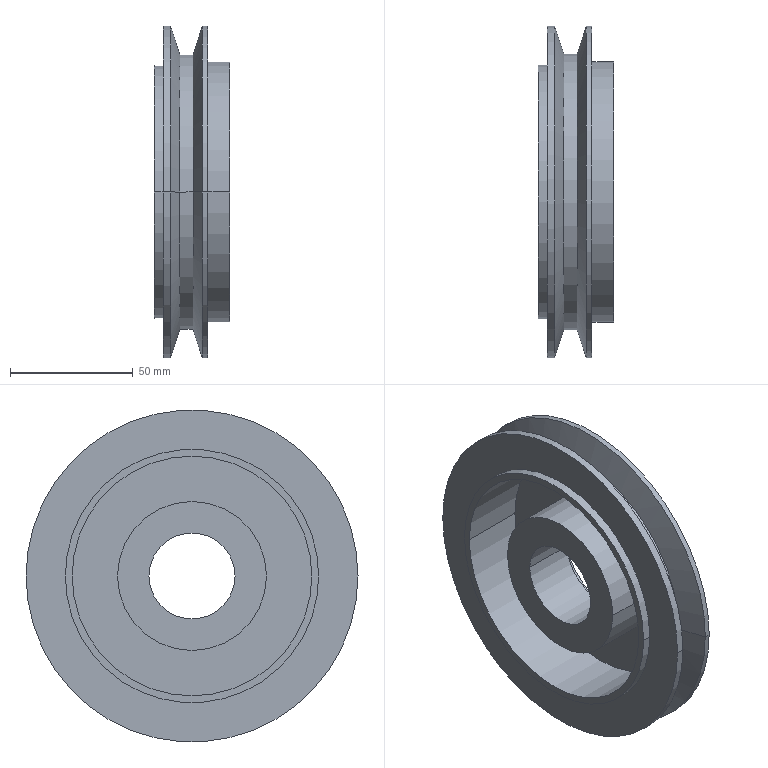Part | STEP file | Market rotor | 1 solid | 29 faces | box 30.5 x 135 x 135 mm | volume 165270 mm3 | cylinder 18 | plane 7 | cone 4 | commonest cylinder face diameters 135 x4 35 x2 48 x2 60.6 x2 97.5 x2 103 x2